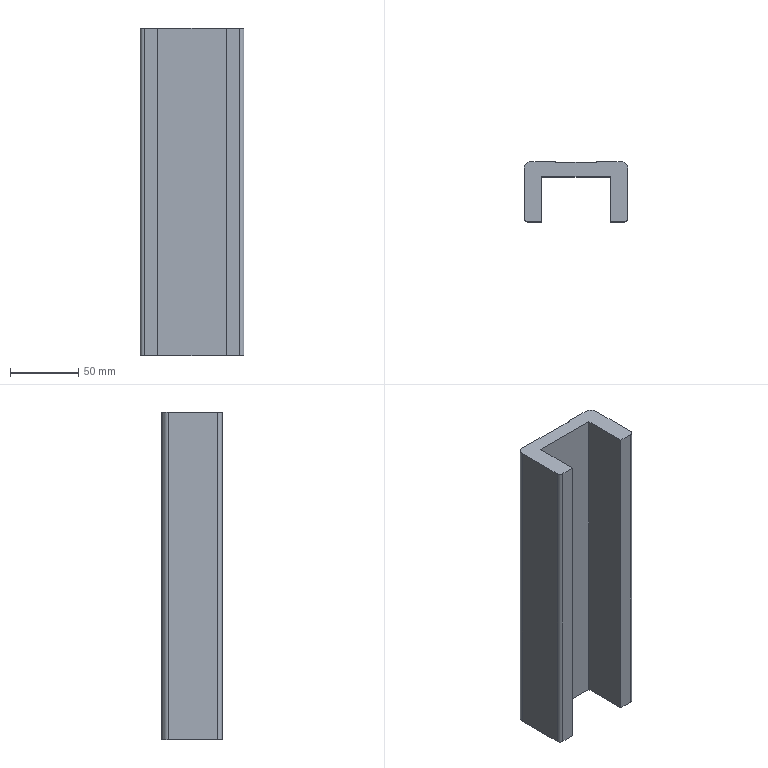Part | SolidWorks | features Cut 1, Extrusion 1 | 1 solid | 54 faces | box 76 x 44 x 240 mm | volume 396756 mm3 | cylinder 28 | plane 26 | commonest cylinder face diameters 5 x16 6 x10 10 x2
STEP:
#1=CARTESIAN_POINT('',(-22.,40.785,-167.));
#2=VERTEX_POINT('',#1);
#3=CARTESIAN_POINT('',(-28.,40.785,-167.));
#4=VERTEX_POINT('',#3);
#5=CARTESIAN_POINT('',(-25.,40.785,-167.));
#6=DIRECTION('',(0.,1.,0.));
#7=DIRECTION('',(-1.,0.,0.));
#8=AXIS2_PLACEMENT_3D('',#5,#6,#7);
#9=CIRCLE('',#8,3.);
#10=EDGE_CURVE('',#2,#4,#9,.T.);
#11=ORIENTED_EDGE('',*,*,#10,.F.);
#12=CARTESIAN_POINT('',(-22.,50.785,-167.));
#13=VERTEX_POINT('',#12);
#14=CARTESIAN_POINT('',(-22.,40.785,-167.));
#15=DIRECTION('',(0.,1.,0.));
#16=VECTOR('',#15,1000.);
#17=LINE('',#14,#16);
#18=EDGE_CURVE('',#2,#13,#17,.T.);
#19=ORIENTED_EDGE('',*,*,#18,.T.);
#20=CARTESIAN_POINT('',(-28.,50.785,-167.));
#21=VERTEX_POINT('',#20);
#22=CARTESIAN_POINT('',(-25.,50.785,-167.));
#23=DIRECTION('',(0.,1.,0.));
#24=DIRECTION('',(-1.,0.,0.));
#25=AXIS2_PLACEMENT_3D('',#22,#23,#24);
#26=CIRCLE('',#25,3.);
#27=EDGE_CURVE('',#13,#21,#26,.T.);
#28=ORIENTED_EDGE('',*,*,#27,.T.);
#29=CARTESIAN_POINT('',(-28.,40.785,-167.));
#30=DIRECTION('',(0.,1.,0.));
#31=VECTOR('',#30,1000.);
#32=LINE('',#29,#31);
#33=EDGE_CURVE('',#4,#21,#32,.T.);
#34=ORIENTED_EDGE('',*,*,#33,.F.);
#35=EDGE_LOOP('',(#11,#19,#28,#34));
#36=FACE_OUTER_BOUND('',#35,.T.);
#37=CARTESIAN_POINT('',(-25.,40.785,-167.));
#38=DIRECTION('',(0.,1.,0.));
#39=DIRECTION('',(-1.,0.,0.));
#40=AXIS2_PLACEMENT_3D('',#37,#38,#39);
#41=CYLINDRICAL_SURFACE('',#40,3.);
#42=ADVANCED_FACE('',(#36),#41,.F.);
#43=CARTESIAN_POINT('',(28.,40.785,-167.));
#44=VERTEX_POINT('',#43);
#45=CARTESIAN_POINT('',(22.,40.785,-167.));
#46=VERTEX_POINT('',#45);
#47=CARTESIAN_POINT('',(25.,40.785,-167.));
#48=DIRECTION('',(0.,1.,0.));
#49=DIRECTION('',(-1.,0.,0.));
#50=AXIS2_PLACEMENT_3D('',#47,#48,#49);
#51=CIRCLE('',#50,3.);
#52=EDGE_CURVE('',#44,#46,#51,.T.);
#53=ORIENTED_EDGE('',*,*,#52,.F.);
#54=CARTESIAN_POINT('',(28.,50.785,-167.));
#55=VERTEX_POINT('',#54);
#56=CARTESIAN_POINT('',(28.,40.785,-167.));
#57=DIRECTION('',(0.,1.,0.));
#58=VECTOR('',#57,1000.);
#59=LINE('',#56,#58);
#60=EDGE_CURVE('',#44,#55,#59,.T.);
#61=ORIENTED_EDGE('',*,*,#60,.T.);
#62=CARTESIAN_POINT('',(22.,50.785,-167.));
#63=VERTEX_POINT('',#62);
#64=CARTESIAN_POINT('',(25.,50.785,-167.));
#65=DIRECTION('',(0.,1.,0.));
#66=DIRECTION('',(-1.,0.,0.));
#67=AXIS2_PLACEMENT_3D('',#64,#65,#66);
#68=CIRCLE('',#67,3.);
#69=EDGE_CURVE('',#55,#63,#68,.T.);
#70=ORIENTED_EDGE('',*,*,#69,.T.);
#71=CARTESIAN_POINT('',(22.,40.785,-167.));
#72=DIRECTION('',(0.,1.,0.));
#73=VECTOR('',#72,1000.);
#74=LINE('',#71,#73);
#75=EDGE_CURVE('',#46,#63,#74,.T.);
#76=ORIENTED_EDGE('',*,*,#75,.F.);
#77=EDGE_LOOP('',(#53,#61,#70,#76));
#78=FACE_OUTER_BOUND('',#77,.T.);
#79=CARTESIAN_POINT('',(25.,40.785,-167.));
#80=DIRECTION('',(0.,1.,0.));
#81=DIRECTION('',(-1.,0.,0.));
#82=AXIS2_PLACEMENT_3D('',#79,#80,#81);
#83=CYLINDRICAL_SURFACE('',#82,3.);
#84=ADVANCED_FACE('',(#78),#83,.F.);
#85=CARTESIAN_POINT('',(-22.,40.785,-73.));
#86=VERTEX_POINT('',#85);
#87=CARTESIAN_POINT('',(-28.,40.785,-73.));
#88=VERTEX_POINT('',#87);
#89=CARTESIAN_POINT('',(-25.,40.785,-73.));
#90=DIRECTION('',(0.,1.,0.));
#91=DIRECTION('',(-1.,0.,0.));
#92=AXIS2_PLACEMENT_3D('',#89,#90,#91);
#93=CIRCLE('',#92,3.);
#94=EDGE_CURVE('',#86,#88,#93,.T.);
#95=ORIENTED_EDGE('',*,*,#94,.F.);
#96=CARTESIAN_POINT('',(-22.,50.785,-73.));
#97=VERTEX_POINT('',#96);
#98=CARTESIAN_POINT('',(-22.,40.785,-73.));
#99=DIRECTION('',(0.,1.,0.));
#100=VECTOR('',#99,1000.);
#101=LINE('',#98,#100);
#102=EDGE_CURVE('',#86,#97,#101,.T.);
#103=ORIENTED_EDGE('',*,*,#102,.T.);
#104=CARTESIAN_POINT('',(-28.,50.785,-73.));
#105=VERTEX_POINT('',#104);
#106=CARTESIAN_POINT('',(-25.,50.785,-73.));
#107=DIRECTION('',(0.,1.,0.));
#108=DIRECTION('',(-1.,0.,0.));
#109=AXIS2_PLACEMENT_3D('',#106,#107,#108);
#110=CIRCLE('',#109,3.);
#111=EDGE_CURVE('',#97,#105,#110,.T.);
#112=ORIENTED_EDGE('',*,*,#111,.T.);
#113=CARTESIAN_POINT('',(-28.,40.785,-73.));
#114=DIRECTION('',(0.,1.,0.));
#115=VECTOR('',#114,1000.);
#116=LINE('',#113,#115);
#117=EDGE_CURVE('',#88,#105,#116,.T.);
#118=ORIENTED_EDGE('',*,*,#117,.F.);
#119=EDGE_LOOP('',(#95,#103,#112,#118));
#120=FACE_OUTER_BOUND('',#119,.T.);
#121=CARTESIAN_POINT('',(-25.,40.785,-73.));
#122=DIRECTION('',(0.,1.,0.));
#123=DIRECTION('',(-1.,0.,0.));
#124=AXIS2_PLACEMENT_3D('',#121,#122,#123);
#125=CYLINDRICAL_SURFACE('',#124,3.);
#126=ADVANCED_FACE('',(#120),#125,.F.);
#127=CARTESIAN_POINT('',(-17.5,40.785,-216.));
#128=VERTEX_POINT('',#127);
#129=CARTESIAN_POINT('',(-22.5,40.785,-216.));
#130=VERTEX_POINT('',#129);
#131=CARTESIAN_POINT('',(-20.,40.785,-216.));
#132=DIRECTION('',(0.,1.,0.));
#133=DIRECTION('',(-1.,0.,0.));
#134=AXIS2_PLACEMENT_3D('',#131,#132,#133);
#135=CIRCLE('',#134,2.5);
#136=EDGE_CURVE('',#128,#130,#135,.T.);
#137=ORIENTED_EDGE('',*,*,#136,.F.);
#138=CARTESIAN_POINT('',(-17.5,50.785,-216.));
#139=VERTEX_POINT('',#138);
#140=CARTESIAN_POINT('',(-17.5,40.785,-216.));
#141=DIRECTION('',(0.,1.,0.));
#142=VECTOR('',#141,1000.);
#143=LINE('',#140,#142);
#144=EDGE_CURVE('',#128,#139,#143,.T.);
#145=ORIENTED_EDGE('',*,*,#144,.T.);
#146=CARTESIAN_POINT('',(-22.5,50.785,-216.));
#147=VERTEX_POINT('',#146);
#148=CARTESIAN_POINT('',(-20.,50.785,-216.));
#149=DIRECTION('',(0.,1.,0.));
#150=DIRECTION('',(-1.,0.,0.));
#151=AXIS2_PLACEMENT_3D('',#148,#149,#150);
#152=CIRCLE('',#151,2.5);
#153=EDGE_CURVE('',#139,#147,#152,.T.);
#154=ORIENTED_EDGE('',*,*,#153,.T.);
#155=CARTESIAN_POINT('',(-22.5,40.785,-216.));
#156=DIRECTION('',(0.,1.,0.));
#157=VECTOR('',#156,1000.);
#158=LINE('',#155,#157);
#159=EDGE_CURVE('',#130,#147,#158,.T.);
#160=ORIENTED_EDGE('',*,*,#159,.F.);
#161=EDGE_LOOP('',(#137,#145,#154,#160));
#162=FACE_OUTER_BOUND('',#161,.T.);
#163=CARTESIAN_POINT('',(-20.,40.785,-216.));
#164=DIRECTION('',(0.,1.,0.));
#165=DIRECTION('',(-1.,0.,0.));
#166=AXIS2_PLACEMENT_3D('',#163,#164,#165);
#167=CYLINDRICAL_SURFACE('',#166,2.5);
#168=ADVANCED_FACE('',(#162),#167,.F.);
#169=CARTESIAN_POINT('',(22.5,40.785,-216.));
#170=VERTEX_POINT('',#169);
#171=CARTESIAN_POINT('',(17.5,40.785,-216.));
#172=VERTEX_POINT('',#171);
#173=CARTESIAN_POINT('',(20.,40.785,-216.));
#174=DIRECTION('',(0.,1.,0.));
#175=DIRECTION('',(-1.,0.,0.));
#176=AXIS2_PLACEMENT_3D('',#173,#174,#175);
#177=CIRCLE('',#176,2.5);
#178=EDGE_CURVE('',#170,#172,#177,.T.);
#179=ORIENTED_EDGE('',*,*,#178,.F.);
#180=CARTESIAN_POINT('',(22.5,50.785,-216.));
#181=VERTEX_POINT('',#180);
#182=CARTESIAN_POINT('',(22.5,40.785,-216.));
#183=DIRECTION('',(0.,1.,0.));
#184=VECTOR('',#183,1000.);
#185=LINE('',#182,#184);
#186=EDGE_CURVE('',#170,#181,#185,.T.);
#187=ORIENTED_EDGE('',*,*,#186,.T.);
#188=CARTESIAN_POINT('',(17.5,50.785,-216.));
#189=VERTEX_POINT('',#188);
#190=CARTESIAN_POINT('',(20.,50.785,-216.));
#191=DIRECTION('',(0.,1.,0.));
#192=DIRECTION('',(-1.,0.,0.));
#193=AXIS2_PLACEMENT_3D('',#190,#191,#192);
#194=CIRCLE('',#193,2.5);
#195=EDGE_CURVE('',#181,#189,#194,.T.);
#196=ORIENTED_EDGE('',*,*,#195,.T.);
#197=CARTESIAN_POINT('',(17.5,40.785,-216.));
#198=DIRECTION('',(0.,1.,0.));
#199=VECTOR('',#198,1000.);
#200=LINE('',#197,#199);
#201=EDGE_CURVE('',#172,#189,#200,.T.);
#202=ORIENTED_EDGE('',*,*,#201,.F.);
#203=EDGE_LOOP('',(#179,#187,#196,#202));
#204=FACE_OUTER_BOUND('',#203,.T.);
#205=CARTESIAN_POINT('',(20.,40.785,-216.));
#206=DIRECTION('',(0.,1.,0.));
#207=DIRECTION('',(-1.,0.,0.));
#208=AXIS2_PLACEMENT_3D('',#205,#206,#207);
#209=CYLINDRICAL_SURFACE('',#208,2.5);
#210=ADVANCED_FACE('',(#204),#209,.F.);
#211=CARTESIAN_POINT('',(-17.5,40.785,-152.));
#212=VERTEX_POINT('',#211);
#213=CARTESIAN_POINT('',(-22.5,40.785,-152.));
#214=VERTEX_POINT('',#213);
#215=CARTESIAN_POINT('',(-20.,40.785,-152.));
#216=DIRECTION('',(0.,1.,0.));
#217=DIRECTION('',(-1.,0.,0.));
#218=AXIS2_PLACEMENT_3D('',#215,#216,#217);
#219=CIRCLE('',#218,2.5);
#220=EDGE_CURVE('',#212,#214,#219,.T.);
#221=ORIENTED_EDGE('',*,*,#220,.F.);
#222=CARTESIAN_POINT('',(-17.5,50.785,-152.));
#223=VERTEX_POINT('',#222);
#224=CARTESIAN_POINT('',(-17.5,40.785,-152.));
#225=DIRECTION('',(0.,1.,0.));
#226=VECTOR('',#225,1000.);
#227=LINE('',#224,#226);
#228=EDGE_CURVE('',#212,#223,#227,.T.);
#229=ORIENTED_EDGE('',*,*,#228,.T.);
#230=CARTESIAN_POINT('',(-22.5,50.785,-152.));
#231=VERTEX_POINT('',#230);
#232=CARTESIAN_POINT('',(-20.,50.785,-152.));
#233=DIRECTION('',(0.,1.,0.));
#234=DIRECTION('',(-1.,0.,0.));
#235=AXIS2_PLACEMENT_3D('',#232,#233,#234);
#236=CIRCLE('',#235,2.5);
#237=EDGE_CURVE('',#223,#231,#236,.T.);
#238=ORIENTED_EDGE('',*,*,#237,.T.);
#239=CARTESIAN_POINT('',(-22.5,40.785,-152.));
#240=DIRECTION('',(0.,1.,0.));
#241=VECTOR('',#240,1000.);
#242=LINE('',#239,#241);
#243=EDGE_CURVE('',#214,#231,#242,.T.);
#244=ORIENTED_EDGE('',*,*,#243,.F.);
#245=EDGE_LOOP('',(#221,#229,#238,#244));
#246=FACE_OUTER_BOUND('',#245,.T.);
#247=CARTESIAN_POINT('',(-20.,40.785,-152.));
#248=DIRECTION('',(0.,1.,0.));
#249=DIRECTION('',(-1.,0.,0.));
#250=AXIS2_PLACEMENT_3D('',#247,#248,#249);
#251=CYLINDRICAL_SURFACE('',#250,2.5);
#252=ADVANCED_FACE('',(#246),#251,.F.);
#253=CARTESIAN_POINT('',(22.5,40.785,-152.));
#254=VERTEX_POINT('',#253);
#255=CARTESIAN_POINT('',(17.5,40.785,-152.));
#256=VERTEX_POINT('',#255);
#257=CARTESIAN_POINT('',(20.,40.785,-152.));
#258=DIRECTION('',(0.,1.,0.));
#259=DIRECTION('',(-1.,0.,0.));
#260=AXIS2_PLACEMENT_3D('',#257,#258,#259);
#261=CIRCLE('',#260,2.5);
#262=EDGE_CURVE('',#254,#256,#261,.T.);
#263=ORIENTED_EDGE('',*,*,#262,.F.);
#264=CARTESIAN_POINT('',(22.5,50.785,-152.));
#265=VERTEX_POINT('',#264);
#266=CARTESIAN_POINT('',(22.5,40.785,-152.));
#267=DIRECTION('',(0.,1.,0.));
#268=VECTOR('',#267,1000.);
#269=LINE('',#266,#268);
#270=EDGE_CURVE('',#254,#265,#269,.T.);
#271=ORIENTED_EDGE('',*,*,#270,.T.);
#272=CARTESIAN_POINT('',(17.5,50.785,-152.));
#273=VERTEX_POINT('',#272);
#274=CARTESIAN_POINT('',(20.,50.785,-152.));
#275=DIRECTION('',(0.,1.,0.));
#276=DIRECTION('',(-1.,0.,0.));
#277=AXIS2_PLACEMENT_3D('',#274,#275,#276);
#278=CIRCLE('',#277,2.5);
#279=EDGE_CURVE('',#265,#273,#278,.T.);
#280=ORIENTED_EDGE('',*,*,#279,.T.);
#281=CARTESIAN_POINT('',(17.5,40.785,-152.));
#282=DIRECTION('',(0.,1.,0.));
#283=VECTOR('',#282,1000.);
#284=LINE('',#281,#283);
#285=EDGE_CURVE('',#256,#273,#284,.T.);
#286=ORIENTED_EDGE('',*,*,#285,.F.);
#287=EDGE_LOOP('',(#263,#271,#280,#286));
#288=FACE_OUTER_BOUND('',#287,.T.);
#289=CARTESIAN_POINT('',(20.,40.785,-152.));
#290=DIRECTION('',(0.,1.,0.));
#291=DIRECTION('',(-1.,0.,0.));
#292=AXIS2_PLACEMENT_3D('',#289,#290,#291);
#293=CYLINDRICAL_SURFACE('',#292,2.5);
#294=ADVANCED_FACE('',(#288),#293,.F.);
#295=CARTESIAN_POINT('',(-17.5,40.785,-88.));
#296=VERTEX_POINT('',#295);
#297=CARTESIAN_POINT('',(-22.5,40.785,-88.));
#298=VERTEX_POINT('',#297);
#299=CARTESIAN_POINT('',(-20.,40.785,-88.));
#300=DIRECTION('',(0.,1.,0.));
#301=DIRECTION('',(-1.,0.,0.));
#302=AXIS2_PLACEMENT_3D('',#299,#300,#301);
#303=CIRCLE('',#302,2.5);
#304=EDGE_CURVE('',#296,#298,#303,.T.);
#305=ORIENTED_EDGE('',*,*,#304,.F.);
#306=CARTESIAN_POINT('',(-17.5,50.785,-88.));
#307=VERTEX_POINT('',#306);
#308=CARTESIAN_POINT('',(-17.5,40.785,-88.));
#309=DIRECTION('',(0.,1.,0.));
#310=VECTOR('',#309,1000.);
#311=LINE('',#308,#310);
#312=EDGE_CURVE('',#296,#307,#311,.T.);
#313=ORIENTED_EDGE('',*,*,#312,.T.);
#314=CARTESIAN_POINT('',(-22.5,50.785,-88.));
#315=VERTEX_POINT('',#314);
#316=CARTESIAN_POINT('',(-20.,50.785,-88.));
#317=DIRECTION('',(0.,1.,0.));
#318=DIRECTION('',(-1.,0.,0.));
#319=AXIS2_PLACEMENT_3D('',#316,#317,#318);
#320=CIRCLE('',#319,2.5);
#321=EDGE_CURVE('',#307,#315,#320,.T.);
#322=ORIENTED_EDGE('',*,*,#321,.T.);
#323=CARTESIAN_POINT('',(-22.5,40.785,-88.));
#324=DIRECTION('',(0.,1.,0.));
#325=VECTOR('',#324,1000.);
#326=LINE('',#323,#325);
#327=EDGE_CURVE('',#298,#315,#326,.T.);
#328=ORIENTED_EDGE('',*,*,#327,.F.);
#329=EDGE_LOOP('',(#305,#313,#322,#328));
#330=FACE_OUTER_BOUND('',#329,.T.);
#331=CARTESIAN_POINT('',(-20.,40.785,-88.));
#332=DIRECTION('',(0.,1.,0.));
#333=DIRECTION('',(-1.,0.,0.));
#334=AXIS2_PLACEMENT_3D('',#331,#332,#333);
#335=CYLINDRICAL_SURFACE('',#334,2.5);
#336=ADVANCED_FACE('',(#330),#335,.F.);
#337=CARTESIAN_POINT('',(22.5,40.785,-88.));
#338=VERTEX_POINT('',#337);
#339=CARTESIAN_POINT('',(17.5,40.785,-88.));
#340=VERTEX_POINT('',#339);
#341=CARTESIAN_POINT('',(20.,40.785,-88.));
#342=DIRECTION('',(0.,1.,0.));
#343=DIRECTION('',(-1.,0.,0.));
#344=AXIS2_PLACEMENT_3D('',#341,#342,#343);
#345=CIRCLE('',#344,2.5);
#346=EDGE_CURVE('',#338,#340,#345,.T.);
#347=ORIENTED_EDGE('',*,*,#346,.F.);
#348=CARTESIAN_POINT('',(22.5,50.785,-88.));
#349=VERTEX_POINT('',#348);
#350=CARTESIAN_POINT('',(22.5,40.785,-88.));
#351=DIRECTION('',(0.,1.,0.));
#352=VECTOR('',#351,1000.);
#353=LINE('',#350,#352);
#354=EDGE_CURVE('',#338,#349,#353,.T.);
#355=ORIENTED_EDGE('',*,*,#354,.T.);
#356=CARTESIAN_POINT('',(17.5,50.785,-88.));
#357=VERTEX_POINT('',#356);
#358=CARTESIAN_POINT('',(20.,50.785,-88.));
#359=DIRECTION('',(0.,1.,0.));
#360=DIRECTION('',(-1.,0.,0.));
#361=AXIS2_PLACEMENT_3D('',#358,#359,#360);
#362=CIRCLE('',#361,2.5);
#363=EDGE_CURVE('',#349,#357,#362,.T.);
#364=ORIENTED_EDGE('',*,*,#363,.T.);
#365=CARTESIAN_POINT('',(17.5,40.785,-88.));
#366=DIRECTION('',(0.,1.,0.));
#367=VECTOR('',#366,1000.);
#368=LINE('',#365,#367);
#369=EDGE_CURVE('',#340,#357,#368,.T.);
#370=ORIENTED_EDGE('',*,*,#369,.F.);
#371=EDGE_LOOP('',(#347,#355,#364,#370));
#372=FACE_OUTER_BOUND('',#371,.T.);
#373=CARTESIAN_POINT('',(20.,40.785,-88.));
#374=DIRECTION('',(0.,1.,0.));
#375=DIRECTION('',(-1.,0.,0.));
#376=AXIS2_PLACEMENT_3D('',#373,#374,#375);
#377=CYLINDRICAL_SURFACE('',#376,2.5);
#378=ADVANCED_FACE('',(#372),#377,.F.);
#379=CARTESIAN_POINT('',(-17.5,40.785,-24.));
#380=VERTEX_POINT('',#379);
#381=CARTESIAN_POINT('',(-22.5,40.785,-24.));
#382=VERTEX_POINT('',#381);
#383=CARTESIAN_POINT('',(-20.,40.785,-24.));
#384=DIRECTION('',(0.,1.,0.));
#385=DIRECTION('',(-1.,0.,0.));
#386=AXIS2_PLACEMENT_3D('',#383,#384,#385);
#387=CIRCLE('',#386,2.5);
#388=EDGE_CURVE('',#380,#382,#387,.T.);
#389=ORIENTED_EDGE('',*,*,#388,.F.);
#390=CARTESIAN_POINT('',(-17.5,50.785,-24.));
#391=VERTEX_POINT('',#390);
#392=CARTESIAN_POINT('',(-17.5,40.785,-24.));
#393=DIRECTION('',(0.,1.,0.));
#394=VECTOR('',#393,1000.);
#395=LINE('',#392,#394);
#396=EDGE_CURVE('',#380,#391,#395,.T.);
#397=ORIENTED_EDGE('',*,*,#396,.T.);
#398=CARTESIAN_POINT('',(-22.5,50.785,-24.));
#399=VERTEX_POINT('',#398);
#400=CARTESIAN_POINT('',(-20.,50.785,-24.));
#401=DIRECTION('',(0.,1.,0.));
#402=DIRECTION('',(-1.,0.,0.));
#403=AXIS2_PLACEMENT_3D('',#400,#401,#402);
#404=CIRCLE('',#403,2.5);
#405=EDGE_CURVE('',#391,#399,#404,.T.);
#406=ORIENTED_EDGE('',*,*,#405,.T.);
#407=CARTESIAN_POINT('',(-22.5,40.785,-24.));
#408=DIRECTION('',(0.,1.,0.));
#409=VECTOR('',#408,1000.);
#410=LINE('',#407,#409);
#411=EDGE_CURVE('',#382,#399,#410,.T.);
#412=ORIENTED_EDGE('',*,*,#411,.F.);
#413=EDGE_LOOP('',(#389,#397,#406,#412));
#414=FACE_OUTER_BOUND('',#413,.T.);
#415=CARTESIAN_POINT('',(-20.,40.785,-24.));
#416=DIRECTION('',(0.,1.,0.));
#417=DIRECTION('',(-1.,0.,0.));
#418=AXIS2_PLACEMENT_3D('',#415,#416,#417);
#419=CYLINDRICAL_SURFACE('',#418,2.5);
#420=ADVANCED_FACE('',(#414),#419,.F.);
#421=CARTESIAN_POINT('',(28.,40.785,-73.));
#422=VERTEX_POINT('',#421);
#423=CARTESIAN_POINT('',(22.,40.785,-73.));
#424=VERTEX_POINT('',#423);
#425=CARTESIAN_POINT('',(25.,40.785,-73.));
#426=DIRECTION('',(0.,1.,0.));
#427=DIRECTION('',(-1.,0.,0.));
#428=AXIS2_PLACEMENT_3D('',#425,#426,#427);
#429=CIRCLE('',#428,3.);
#430=EDGE_CURVE('',#422,#424,#429,.T.);
#431=ORIENTED_EDGE('',*,*,#430,.F.);
#432=CARTESIAN_POINT('',(28.,50.785,-73.));
#433=VERTEX_POINT('',#432);
#434=CARTESIAN_POINT('',(28.,40.785,-73.));
#435=DIRECTION('',(0.,1.,0.));
#436=VECTOR('',#435,1000.);
#437=LINE('',#434,#436);
#438=EDGE_CURVE('',#422,#433,#437,.T.);
#439=ORIENTED_EDGE('',*,*,#438,.T.);
#440=CARTESIAN_POINT('',(22.,50.785,-73.));
#441=VERTEX_POINT('',#440);
#442=CARTESIAN_POINT('',(25.,50.785,-73.));
#443=DIRECTION('',(0.,1.,0.));
#444=DIRECTION('',(-1.,0.,0.));
#445=AXIS2_PLACEMENT_3D('',#442,#443,#444);
#446=CIRCLE('',#445,3.);
#447=EDGE_CURVE('',#433,#441,#446,.T.);
#448=ORIENTED_EDGE('',*,*,#447,.T.);
#449=CARTESIAN_POINT('',(22.,40.785,-73.));
#450=DIRECTION('',(0.,1.,0.));
#451=VECTOR('',#450,1000.);
#452=LINE('',#449,#451);
#453=EDGE_CURVE('',#424,#441,#452,.T.);
#454=ORIENTED_EDGE('',*,*,#453,.F.);
#455=EDGE_LOOP('',(#431,#439,#448,#454));
#456=FACE_OUTER_BOUND('',#455,.T.);
#457=CARTESIAN_POINT('',(25.,40.785,-73.));
#458=DIRECTION('',(0.,1.,0.));
#459=DIRECTION('',(-1.,0.,0.));
#460=AXIS2_PLACEMENT_3D('',#457,#458,#459);
#461=CYLINDRICAL_SURFACE('',#460,3.);
#462=ADVANCED_FACE('',(#456),#461,.F.);
#463=CARTESIAN_POINT('',(22.5,40.785,-24.));
#464=VERTEX_POINT('',#463);
#465=CARTESIAN_POINT('',(17.5,40.785,-24.));
#466=VERTEX_POINT('',#465);
#467=CARTESIAN_POINT('',(20.,40.785,-24.));
#468=DIRECTION('',(0.,1.,0.));
#469=DIRECTION('',(-1.,0.,0.));
#470=AXIS2_PLACEMENT_3D('',#467,#468,#469);
#471=CIRCLE('',#470,2.5);
#472=EDGE_CURVE('',#464,#466,#471,.T.);
#473=ORIENTED_EDGE('',*,*,#472,.F.);
#474=CARTESIAN_POINT('',(22.5,50.785,-24.));
#475=VERTEX_POINT('',#474);
#476=CARTESIAN_POINT('',(22.5,40.785,-24.));
#477=DIRECTION('',(0.,1.,0.));
#478=VECTOR('',#477,1000.);
#479=LINE('',#476,#478);
#480=EDGE_CURVE('',#464,#475,#479,.T.);
#481=ORIENTED_EDGE('',*,*,#480,.T.);
#482=CARTESIAN_POINT('',(17.5,50.785,-24.));
#483=VERTEX_POINT('',#482);
#484=CARTESIAN_POINT('',(20.,50.785,-24.));
#485=DIRECTION('',(0.,1.,0.));
#486=DIRECTION('',(-1.,0.,0.));
#487=AXIS2_PLACEMENT_3D('',#484,#485,#486);
#488=CIRCLE('',#487,2.5);
#489=EDGE_CURVE('',#475,#483,#488,.T.);
#490=ORIENTED_EDGE('',*,*,#489,.T.);
#491=CARTESIAN_POINT('',(17.5,40.785,-24.));
#492=DIRECTION('',(0.,1.,0.));
#493=VECTOR('',#492,1000.);
#494=LINE('',#491,#493);
#495=EDGE_CURVE('',#466,#483,#494,.T.);
#496=ORIENTED_EDGE('',*,*,#495,.F.);
#497=EDGE_LOOP('',(#473,#481,#490,#496));
#498=FACE_OUTER_BOUND('',#497,.T.);
#499=CARTESIAN_POINT('',(20.,40.785,-24.));
#500=DIRECTION('',(0.,1.,0.));
#501=DIRECTION('',(-1.,0.,0.));
#502=AXIS2_PLACEMENT_3D('',#499,#500,#501);
#503=CYLINDRICAL_SURFACE('',#502,2.5);
#504=ADVANCED_FACE('',(#498),#503,.F.);
#505=CARTESIAN_POINT('',(-25.,50.785,-167.));
#506=DIRECTION('',(0.,1.,0.));
#507=DIRECTION('',(-1.,0.,0.));
#508=AXIS2_PLACEMENT_3D('',#505,#506,#507);
#509=CIRCLE('',#508,3.);
#510=EDGE_CURVE('',#21,#13,#509,.T.);
#511=ORIENTED_EDGE('',*,*,#510,.F.);
#512=ORIENTED_EDGE('',*,*,#27,.F.);
#513=EDGE_LOOP('',(#511,#512));
#514=FACE_BOUND('',#513,.T.);
#515=CARTESIAN_POINT('',(-25.,50.785,-73.));
#516=DIRECTION('',(0.,1.,0.));
#517=DIRECTION('',(-1.,0.,0.));
#518=AXIS2_PLACEMENT_3D('',#515,#516,#517);
#519=CIRCLE('',#518,3.);
#520=EDGE_CURVE('',#105,#97,#519,.T.);
#521=ORIENTED_EDGE('',*,*,#520,.F.);
#522=ORIENTED_EDGE('',*,*,#111,.F.);
#523=EDGE_LOOP('',(#521,#522));
#524=FACE_BOUND('',#523,.T.);
#525=CARTESIAN_POINT('',(-20.,50.785,-216.));
#526=DIRECTION('',(0.,1.,0.));
#527=DIRECTION('',(-1.,0.,0.));
#528=AXIS2_PLACEMENT_3D('',#525,#526,#527);
#529=CIRCLE('',#528,2.5);
#530=EDGE_CURVE('',#147,#139,#529,.T.);
#531=ORIENTED_EDGE('',*,*,#530,.F.);
#532=ORIENTED_EDGE('',*,*,#153,.F.);
#533=EDGE_LOOP('',(#531,#532));
#534=FACE_BOUND('',#533,.T.);
#535=CARTESIAN_POINT('',(-20.,50.785,-152.));
#536=DIRECTION('',(0.,1.,0.));
#537=DIRECTION('',(-1.,0.,0.));
#538=AXIS2_PLACEMENT_3D('',#535,#536,#537);
#539=CIRCLE('',#538,2.5);
#540=EDGE_CURVE('',#231,#223,#539,.T.);
#541=ORIENTED_EDGE('',*,*,#540,.F.);
#542=ORIENTED_EDGE('',*,*,#237,.F.);
#543=EDGE_LOOP('',(#541,#542));
#544=FACE_BOUND('',#543,.T.);
#545=CARTESIAN_POINT('',(-20.,50.785,-88.));
#546=DIRECTION('',(0.,1.,0.));
#547=DIRECTION('',(-1.,0.,0.));
#548=AXIS2_PLACEMENT_3D('',#545,#546,#547);
#549=CIRCLE('',#548,2.5);
#550=EDGE_CURVE('',#315,#307,#549,.T.);
#551=ORIENTED_EDGE('',*,*,#550,.F.);
#552=ORIENTED_EDGE('',*,*,#321,.F.);
#553=EDGE_LOOP('',(#551,#552));
#554=FACE_BOUND('',#553,.T.);
#555=CARTESIAN_POINT('',(-20.,50.785,-24.));
#556=DIRECTION('',(0.,1.,0.));
#557=DIRECTION('',(-1.,0.,0.));
#558=AXIS2_PLACEMENT_3D('',#555,#556,#557);
#559=CIRCLE('',#558,2.5);
#560=EDGE_CURVE('',#399,#391,#559,.T.);
#561=ORIENTED_EDGE('',*,*,#560,.F.);
#562=ORIENTED_EDGE('',*,*,#405,.F.);
#563=EDGE_LOOP('',(#561,#562));
#564=FACE_BOUND('',#563,.T.);
#565=CARTESIAN_POINT('',(-15.,50.785,0.));
#566=VERTEX_POINT('',#565);
#567=CARTESIAN_POINT('',(-33.,50.785,0.));
#568=VERTEX_POINT('',#567);
#569=CARTESIAN_POINT('',(-15.,50.785,0.));
#570=DIRECTION('',(-1.,0.,0.));
#571=VECTOR('',#570,1000.);
#572=LINE('',#569,#571);
#573=EDGE_CURVE('',#566,#568,#572,.T.);
#574=ORIENTED_EDGE('',*,*,#573,.F.);
#575=CARTESIAN_POINT('',(-15.,50.785,-240.));
#576=VERTEX_POINT('',#575);
#577=CARTESIAN_POINT('',(-15.,50.785,-240.));
#578=DIRECTION('',(0.,0.,1.));
#579=VECTOR('',#578,1000.);
#580=LINE('',#577,#579);
#581=EDGE_CURVE('',#576,#566,#580,.T.);
#582=ORIENTED_EDGE('',*,*,#581,.F.);
#583=CARTESIAN_POINT('',(-33.,50.785,-240.));
#584=VERTEX_POINT('',#583);
#585=CARTESIAN_POINT('',(-15.,50.785,-240.));
#586=DIRECTION('',(-1.,0.,0.));
#587=VECTOR('',#586,1000.);
#588=LINE('',#585,#587);
#589=EDGE_CURVE('',#576,#584,#588,.T.);
#590=ORIENTED_EDGE('',*,*,#589,.T.);
#591=CARTESIAN_POINT('',(-33.,50.785,-240.));
#592=DIRECTION('',(0.,0.,1.));
#593=VECTOR('',#592,1000.);
#594=LINE('',#591,#593);
#595=EDGE_CURVE('',#584,#568,#594,.T.);
#596=ORIENTED_EDGE('',*,*,#595,.T.);
#597=EDGE_LOOP('',(#574,#582,#590,#596));
#598=FACE_OUTER_BOUND('',#597,.T.);
#599=CARTESIAN_POINT('',(-15.,50.785,-240.));
#600=DIRECTION('',(0.,1.,0.));
#601=DIRECTION('',(-1.,0.,0.));
#602=AXIS2_PLACEMENT_3D('',#599,#600,#601);
#603=PLANE('',#602);
#604=ADVANCED_FACE('',(#514,#524,#534,#544,#554,#564,#598),#603,.T.);
#605=CARTESIAN_POINT('',(-15.,50.285,0.));
#606=VERTEX_POINT('',#605);
#607=CARTESIAN_POINT('',(-15.,50.785,0.));
#608=DIRECTION('',(0.,1.,0.));
#609=VECTOR('',#608,1000.);
#610=LINE('',#607,#609);
#611=EDGE_CURVE('',#606,#566,#610,.T.);
#612=ORIENTED_EDGE('',*,*,#611,.F.);
#613=CARTESIAN_POINT('',(-15.,50.285,-240.));
#614=VERTEX_POINT('',#613);
#615=CARTESIAN_POINT('',(-15.,50.285,-240.));
#616=DIRECTION('',(0.,0.,1.));
#617=VECTOR('',#616,1000.);
#618=LINE('',#615,#617);
#619=EDGE_CURVE('',#614,#606,#618,.T.);
#620=ORIENTED_EDGE('',*,*,#619,.F.);
#621=CARTESIAN_POINT('',(-15.,50.785,-240.));
#622=DIRECTION('',(0.,1.,0.));
#623=VECTOR('',#622,1000.);
#624=LINE('',#621,#623);
#625=EDGE_CURVE('',#614,#576,#624,.T.);
#626=ORIENTED_EDGE('',*,*,#625,.T.);
#627=ORIENTED_EDGE('',*,*,#581,.T.);
#628=EDGE_LOOP('',(#612,#620,#626,#627));
#629=FACE_OUTER_BOUND('',#628,.T.);
#630=CARTESIAN_POINT('',(-15.,50.785,-240.));
#631=DIRECTION('',(1.,0.,0.));
#632=DIRECTION('',(0.,0.,-1.));
#633=AXIS2_PLACEMENT_3D('',#630,#631,#632);
#634=PLANE('',#633);
#635=ADVANCED_FACE('',(#629),#634,.T.);
#636=CARTESIAN_POINT('',(15.,50.285,0.));
#637=VERTEX_POINT('',#636);
#638=CARTESIAN_POINT('',(-15.,50.285,0.));
#639=DIRECTION('',(-1.,0.,0.));
#640=VECTOR('',#639,1000.);
#641=LINE('',#638,#640);
#642=EDGE_CURVE('',#637,#606,#641,.T.);
#643=ORIENTED_EDGE('',*,*,#642,.F.);
#644=CARTESIAN_POINT('',(15.,50.285,-240.));
#645=VERTEX_POINT('',#644);
#646=CARTESIAN_POINT('',(15.,50.285,-240.));
#647=DIRECTION('',(0.,0.,1.));
#648=VECTOR('',#647,1000.);
#649=LINE('',#646,#648);
#650=EDGE_CURVE('',#645,#637,#649,.T.);
#651=ORIENTED_EDGE('',*,*,#650,.F.);
#652=CARTESIAN_POINT('',(-15.,50.285,-240.));
#653=DIRECTION('',(-1.,0.,0.));
#654=VECTOR('',#653,1000.);
#655=LINE('',#652,#654);
#656=EDGE_CURVE('',#645,#614,#655,.T.);
#657=ORIENTED_EDGE('',*,*,#656,.T.);
#658=ORIENTED_EDGE('',*,*,#619,.T.);
#659=EDGE_LOOP('',(#643,#651,#657,#658));
#660=FACE_OUTER_BOUND('',#659,.T.);
#661=CARTESIAN_POINT('',(-15.,50.285,-240.));
#662=DIRECTION('',(0.,1.,0.));
#663=DIRECTION('',(0.,0.,1.));
#664=AXIS2_PLACEMENT_3D('',#661,#662,#663);
#665=PLANE('',#664);
#666=ADVANCED_FACE('',(#660),#665,.T.);
#667=CARTESIAN_POINT('',(15.,50.785,0.));
#668=VERTEX_POINT('',#667);
#669=CARTESIAN_POINT('',(15.,50.785,0.));
#670=DIRECTION('',(0.,-1.,0.));
#671=VECTOR('',#670,1000.);
#672=LINE('',#669,#671);
#673=EDGE_CURVE('',#668,#637,#672,.T.);
#674=ORIENTED_EDGE('',*,*,#673,.F.);
#675=CARTESIAN_POINT('',(15.,50.785,-240.));
#676=VERTEX_POINT('',#675);
#677=CARTESIAN_POINT('',(15.,50.785,-240.));
#678=DIRECTION('',(0.,0.,1.));
#679=VECTOR('',#678,1000.);
#680=LINE('',#677,#679);
#681=EDGE_CURVE('',#676,#668,#680,.T.);
#682=ORIENTED_EDGE('',*,*,#681,.F.);
#683=CARTESIAN_POINT('',(15.,50.785,-240.));
#684=DIRECTION('',(0.,-1.,0.));
#685=VECTOR('',#684,1000.);
#686=LINE('',#683,#685);
#687=EDGE_CURVE('',#676,#645,#686,.T.);
#688=ORIENTED_EDGE('',*,*,#687,.T.);
#689=ORIENTED_EDGE('',*,*,#650,.T.);
#690=EDGE_LOOP('',(#674,#682,#688,#689));
#691=FACE_OUTER_BOUND('',#690,.T.);
#692=CARTESIAN_POINT('',(15.,50.785,-240.));
#693=DIRECTION('',(-1.,0.,0.));
#694=DIRECTION('',(0.,0.,1.));
#695=AXIS2_PLACEMENT_3D('',#692,#693,#694);
#696=PLANE('',#695);
#697=ADVANCED_FACE('',(#691),#696,.T.);
#698=CARTESIAN_POINT('',(25.,50.785,-167.));
#699=DIRECTION('',(0.,1.,0.));
#700=DIRECTION('',(-1.,0.,0.));
#701=AXIS2_PLACEMENT_3D('',#698,#699,#700);
#702=CIRCLE('',#701,3.);
#703=EDGE_CURVE('',#63,#55,#702,.T.);
#704=ORIENTED_EDGE('',*,*,#703,.F.);
#705=ORIENTED_EDGE('',*,*,#69,.F.);
#706=EDGE_LOOP('',(#704,#705));
#707=FACE_BOUND('',#706,.T.);
#708=CARTESIAN_POINT('',(20.,50.785,-216.));
#709=DIRECTION('',(0.,1.,0.));
#710=DIRECTION('',(-1.,0.,0.));
#711=AXIS2_PLACEMENT_3D('',#708,#709,#710);
#712=CIRCLE('',#711,2.5);
#713=EDGE_CURVE('',#189,#181,#712,.T.);
#714=ORIENTED_EDGE('',*,*,#713,.F.);
#715=ORIENTED_EDGE('',*,*,#195,.F.);
#716=EDGE_LOOP('',(#714,#715));
#717=FACE_BOUND('',#716,.T.);
#718=CARTESIAN_POINT('',(20.,50.785,-152.));
#719=DIRECTION('',(0.,1.,0.));
#720=DIRECTION('',(-1.,0.,0.));
#721=AXIS2_PLACEMENT_3D('',#718,#719,#720);
#722=CIRCLE('',#721,2.5);
#723=EDGE_CURVE('',#273,#265,#722,.T.);
#724=ORIENTED_EDGE('',*,*,#723,.F.);
#725=ORIENTED_EDGE('',*,*,#279,.F.);
#726=EDGE_LOOP('',(#724,#725));
#727=FACE_BOUND('',#726,.T.);
#728=CARTESIAN_POINT('',(20.,50.785,-88.));
#729=DIRECTION('',(0.,1.,0.));
#730=DIRECTION('',(-1.,0.,0.));
#731=AXIS2_PLACEMENT_3D('',#728,#729,#730);
#732=CIRCLE('',#731,2.5);
#733=EDGE_CURVE('',#357,#349,#732,.T.);
#734=ORIENTED_EDGE('',*,*,#733,.F.);
#735=ORIENTED_EDGE('',*,*,#363,.F.);
#736=EDGE_LOOP('',(#734,#735));
#737=FACE_BOUND('',#736,.T.);
#738=CARTESIAN_POINT('',(25.,50.785,-73.));
#739=DIRECTION('',(0.,1.,0.));
#740=DIRECTION('',(-1.,0.,0.));
#741=AXIS2_PLACEMENT_3D('',#738,#739,#740);
#742=CIRCLE('',#741,3.);
#743=EDGE_CURVE('',#441,#433,#742,.T.);
#744=ORIENTED_EDGE('',*,*,#743,.F.);
#745=ORIENTED_EDGE('',*,*,#447,.F.);
#746=EDGE_LOOP('',(#744,#745));
#747=FACE_BOUND('',#746,.T.);
#748=CARTESIAN_POINT('',(20.,50.785,-24.));
#749=DIRECTION('',(0.,1.,0.));
#750=DIRECTION('',(-1.,0.,0.));
#751=AXIS2_PLACEMENT_3D('',#748,#749,#750);
#752=CIRCLE('',#751,2.5);
#753=EDGE_CURVE('',#483,#475,#752,.T.);
#754=ORIENTED_EDGE('',*,*,#753,.F.);
#755=ORIENTED_EDGE('',*,*,#489,.F.);
#756=EDGE_LOOP('',(#754,#755));
#757=FACE_BOUND('',#756,.T.);
#758=CARTESIAN_POINT('',(33.,50.785,0.));
#759=VERTEX_POINT('',#758);
#760=CARTESIAN_POINT('',(33.,50.785,0.));
#761=DIRECTION('',(-1.,0.,0.));
#762=VECTOR('',#761,1000.);
#763=LINE('',#760,#762);
#764=EDGE_CURVE('',#759,#668,#763,.T.);
#765=ORIENTED_EDGE('',*,*,#764,.F.);
#766=CARTESIAN_POINT('',(33.,50.785,-240.));
#767=VERTEX_POINT('',#766);
#768=CARTESIAN_POINT('',(33.,50.785,-240.));
#769=DIRECTION('',(0.,0.,1.));
#770=VECTOR('',#769,1000.);
#771=LINE('',#768,#770);
#772=EDGE_CURVE('',#767,#759,#771,.T.);
#773=ORIENTED_EDGE('',*,*,#772,.F.);
#774=CARTESIAN_POINT('',(33.,50.785,-240.));
#775=DIRECTION('',(-1.,0.,0.));
#776=VECTOR('',#775,1000.);
#777=LINE('',#774,#776);
#778=EDGE_CURVE('',#767,#676,#777,.T.);
#779=ORIENTED_EDGE('',*,*,#778,.T.);
#780=ORIENTED_EDGE('',*,*,#681,.T.);
#781=EDGE_LOOP('',(#765,#773,#779,#780));
#782=FACE_OUTER_BOUND('',#781,.T.);
#783=CARTESIAN_POINT('',(33.,50.785,-240.));
#784=DIRECTION('',(0.,1.,0.));
#785=DIRECTION('',(-1.,0.,0.));
#786=AXIS2_PLACEMENT_3D('',#783,#784,#785);
#787=PLANE('',#786);
#788=ADVANCED_FACE('',(#707,#717,#727,#737,#747,#757,#782),#787,.T.);
#789=CARTESIAN_POINT('',(38.,45.785,0.));
#790=VERTEX_POINT('',#789);
#791=CARTESIAN_POINT('',(33.,45.785,0.));
#792=DIRECTION('',(0.,0.,1.));
#793=DIRECTION('',(1.,0.,0.));
#794=AXIS2_PLACEMENT_3D('',#791,#792,#793);
#795=CIRCLE('',#794,5.);
#796=EDGE_CURVE('',#790,#759,#795,.T.);
#797=ORIENTED_EDGE('',*,*,#796,.F.);
#798=CARTESIAN_POINT('',(38.,45.785,-240.));
#799=VERTEX_POINT('',#798);
#800=CARTESIAN_POINT('',(38.,45.785,-240.));
#801=DIRECTION('',(0.,0.,1.));
#802=VECTOR('',#801,1000.);
#803=LINE('',#800,#802);
#804=EDGE_CURVE('',#799,#790,#803,.T.);
#805=ORIENTED_EDGE('',*,*,#804,.F.);
#806=CARTESIAN_POINT('',(33.,45.785,-240.));
#807=DIRECTION('',(0.,0.,1.));
#808=DIRECTION('',(1.,0.,0.));
#809=AXIS2_PLACEMENT_3D('',#806,#807,#808);
#810=CIRCLE('',#809,5.);
#811=EDGE_CURVE('',#799,#767,#810,.T.);
#812=ORIENTED_EDGE('',*,*,#811,.T.);
#813=ORIENTED_EDGE('',*,*,#772,.T.);
#814=EDGE_LOOP('',(#797,#805,#812,#813));
#815=FACE_OUTER_BOUND('',#814,.T.);
#816=CARTESIAN_POINT('',(33.,45.785,-240.));
#817=DIRECTION('',(0.,0.,1.));
#818=DIRECTION('',(1.,0.,0.));
#819=AXIS2_PLACEMENT_3D('',#816,#817,#818);
#820=CYLINDRICAL_SURFACE('',#819,5.);
#821=ADVANCED_FACE('',(#815),#820,.T.);
#822=CARTESIAN_POINT('',(38.,9.785,0.));
#823=VERTEX_POINT('',#822);
#824=CARTESIAN_POINT('',(38.,45.785,0.));
#825=DIRECTION('',(0.,1.,0.));
#826=VECTOR('',#825,1000.);
#827=LINE('',#824,#826);
#828=EDGE_CURVE('',#823,#790,#827,.T.);
#829=ORIENTED_EDGE('',*,*,#828,.F.);
#830=CARTESIAN_POINT('',(38.,9.785,-240.));
#831=VERTEX_POINT('',#830);
#832=CARTESIAN_POINT('',(38.,9.785,-240.));
#833=DIRECTION('',(0.,0.,1.));
#834=VECTOR('',#833,1000.);
#835=LINE('',#832,#834);
#836=EDGE_CURVE('',#831,#823,#835,.T.);
#837=ORIENTED_EDGE('',*,*,#836,.F.);
#838=CARTESIAN_POINT('',(38.,45.785,-240.));
#839=DIRECTION('',(0.,1.,0.));
#840=VECTOR('',#839,1000.);
#841=LINE('',#838,#840);
#842=EDGE_CURVE('',#831,#799,#841,.T.);
#843=ORIENTED_EDGE('',*,*,#842,.T.);
#844=ORIENTED_EDGE('',*,*,#804,.T.);
#845=EDGE_LOOP('',(#829,#837,#843,#844));
#846=FACE_OUTER_BOUND('',#845,.T.);
#847=CARTESIAN_POINT('',(38.,45.785,-240.));
#848=DIRECTION('',(1.,0.,0.));
#849=DIRECTION('',(0.,1.,0.));
#850=AXIS2_PLACEMENT_3D('',#847,#848,#849);
#851=PLANE('',#850);
#852=ADVANCED_FACE('',(#846),#851,.T.);
#853=CARTESIAN_POINT('',(35.,6.785,0.));
#854=VERTEX_POINT('',#853);
#855=CARTESIAN_POINT('',(35.,9.785,0.));
#856=DIRECTION('',(0.,0.,1.));
#857=DIRECTION('',(-1.,0.,0.));
#858=AXIS2_PLACEMENT_3D('',#855,#856,#857);
#859=CIRCLE('',#858,3.);
#860=EDGE_CURVE('',#854,#823,#859,.T.);
#861=ORIENTED_EDGE('',*,*,#860,.F.);
#862=CARTESIAN_POINT('',(35.,6.785,-240.));
#863=VERTEX_POINT('',#862);
#864=CARTESIAN_POINT('',(35.,6.785,-240.));
#865=DIRECTION('',(0.,0.,1.));
#866=VECTOR('',#865,1000.);
#867=LINE('',#864,#866);
#868=EDGE_CURVE('',#863,#854,#867,.T.);
#869=ORIENTED_EDGE('',*,*,#868,.F.);
#870=CARTESIAN_POINT('',(35.,9.785,-240.));
#871=DIRECTION('',(0.,0.,1.));
#872=DIRECTION('',(-1.,0.,0.));
#873=AXIS2_PLACEMENT_3D('',#870,#871,#872);
#874=CIRCLE('',#873,3.);
#875=EDGE_CURVE('',#863,#831,#874,.T.);
#876=ORIENTED_EDGE('',*,*,#875,.T.);
#877=ORIENTED_EDGE('',*,*,#836,.T.);
#878=EDGE_LOOP('',(#861,#869,#876,#877));
#879=FACE_OUTER_BOUND('',#878,.T.);
#880=CARTESIAN_POINT('',(35.,9.785,-240.));
#881=DIRECTION('',(0.,0.,1.));
#882=DIRECTION('',(1.,0.,0.));
#883=AXIS2_PLACEMENT_3D('',#880,#881,#882);
#884=CYLINDRICAL_SURFACE('',#883,3.);
#885=ADVANCED_FACE('',(#879),#884,.T.);
#886=CARTESIAN_POINT('',(25.,6.785,0.));
#887=VERTEX_POINT('',#886);
#888=CARTESIAN_POINT('',(35.,6.785,0.));
#889=DIRECTION('',(1.,0.,0.));
#890=VECTOR('',#889,1000.);
#891=LINE('',#888,#890);
#892=EDGE_CURVE('',#887,#854,#891,.T.);
#893=ORIENTED_EDGE('',*,*,#892,.F.);
#894=CARTESIAN_POINT('',(25.,6.785,-240.));
#895=VERTEX_POINT('',#894);
#896=CARTESIAN_POINT('',(25.,6.785,-240.));
#897=DIRECTION('',(0.,0.,1.));
#898=VECTOR('',#897,1000.);
#899=LINE('',#896,#898);
#900=EDGE_CURVE('',#895,#887,#899,.T.);
#901=ORIENTED_EDGE('',*,*,#900,.F.);
#902=CARTESIAN_POINT('',(35.,6.785,-240.));
#903=DIRECTION('',(1.,0.,0.));
#904=VECTOR('',#903,1000.);
#905=LINE('',#902,#904);
#906=EDGE_CURVE('',#895,#863,#905,.T.);
#907=ORIENTED_EDGE('',*,*,#906,.T.);
#908=ORIENTED_EDGE('',*,*,#868,.T.);
#909=EDGE_LOOP('',(#893,#901,#907,#908));
#910=FACE_OUTER_BOUND('',#909,.T.);
#911=CARTESIAN_POINT('',(35.,6.785,-240.));
#912=DIRECTION('',(0.,-1.,0.));
#913=DIRECTION('',(0.,0.,-1.));
#914=AXIS2_PLACEMENT_3D('',#911,#912,#913);
#915=PLANE('',#914);
#916=ADVANCED_FACE('',(#910),#915,.T.);
#917=CARTESIAN_POINT('',(25.,39.785,0.));
#918=VERTEX_POINT('',#917);
#919=CARTESIAN_POINT('',(25.,6.785,0.));
#920=DIRECTION('',(0.,-1.,0.));
#921=VECTOR('',#920,1000.);
#922=LINE('',#919,#921);
#923=EDGE_CURVE('',#918,#887,#922,.T.);
#924=ORIENTED_EDGE('',*,*,#923,.F.);
#925=CARTESIAN_POINT('',(25.,39.785,-240.));
#926=VERTEX_POINT('',#925);
#927=CARTESIAN_POINT('',(25.,39.785,-240.));
#928=DIRECTION('',(0.,0.,1.));
#929=VECTOR('',#928,1000.);
#930=LINE('',#927,#929);
#931=EDGE_CURVE('',#926,#918,#930,.T.);
#932=ORIENTED_EDGE('',*,*,#931,.F.);
#933=CARTESIAN_POINT('',(25.,6.785,-240.));
#934=DIRECTION('',(0.,-1.,0.));
#935=VECTOR('',#934,1000.);
#936=LINE('',#933,#935);
#937=EDGE_CURVE('',#926,#895,#936,.T.);
#938=ORIENTED_EDGE('',*,*,#937,.T.);
#939=ORIENTED_EDGE('',*,*,#900,.T.);
#940=EDGE_LOOP('',(#924,#932,#938,#939));
#941=FACE_OUTER_BOUND('',#940,.T.);
#942=CARTESIAN_POINT('',(25.,6.785,-240.));
#943=DIRECTION('',(-1.,0.,0.));
#944=DIRECTION('',(0.,0.,1.));
#945=AXIS2_PLACEMENT_3D('',#942,#943,#944);
#946=PLANE('',#945);
#947=ADVANCED_FACE('',(#941),#946,.T.);
#948=CARTESIAN_POINT('',(-25.,39.785,0.));
#949=VERTEX_POINT('',#948);
#950=CARTESIAN_POINT('',(-25.,39.785,0.));
#951=DIRECTION('',(1.,0.,0.));
#952=VECTOR('',#951,1000.);
#953=LINE('',#950,#952);
#954=EDGE_CURVE('',#949,#918,#953,.T.);
#955=ORIENTED_EDGE('',*,*,#954,.F.);
#956=CARTESIAN_POINT('',(-25.,39.785,-240.));
#957=VERTEX_POINT('',#956);
#958=CARTESIAN_POINT('',(-25.,39.785,-240.));
#959=DIRECTION('',(0.,0.,1.));
#960=VECTOR('',#959,1000.);
#961=LINE('',#958,#960);
#962=EDGE_CURVE('',#957,#949,#961,.T.);
#963=ORIENTED_EDGE('',*,*,#962,.F.);
#964=CARTESIAN_POINT('',(-25.,39.785,-240.));
#965=DIRECTION('',(1.,0.,0.));
#966=VECTOR('',#965,1000.);
#967=LINE('',#964,#966);
#968=EDGE_CURVE('',#957,#926,#967,.T.);
#969=ORIENTED_EDGE('',*,*,#968,.T.);
#970=ORIENTED_EDGE('',*,*,#931,.T.);
#971=EDGE_LOOP('',(#955,#963,#969,#970));
#972=FACE_OUTER_BOUND('',#971,.T.);
#973=CARTESIAN_POINT('',(-25.,39.785,-240.));
#974=DIRECTION('',(0.,-1.,0.));
#975=DIRECTION('',(0.,0.,-1.));
#976=AXIS2_PLACEMENT_3D('',#973,#974,#975);
#977=PLANE('',#976);
#978=ADVANCED_FACE('',(#972),#977,.T.);
#979=CARTESIAN_POINT('',(-25.,6.785,0.));
#980=VERTEX_POINT('',#979);
#981=CARTESIAN_POINT('',(-25.,6.785,0.));
#982=DIRECTION('',(0.,1.,0.));
#983=VECTOR('',#982,1000.);
#984=LINE('',#981,#983);
#985=EDGE_CURVE('',#980,#949,#984,.T.);
#986=ORIENTED_EDGE('',*,*,#985,.F.);
#987=CARTESIAN_POINT('',(-25.,6.785,-240.));
#988=VERTEX_POINT('',#987);
#989=CARTESIAN_POINT('',(-25.,6.785,-240.));
#990=DIRECTION('',(0.,0.,1.));
#991=VECTOR('',#990,1000.);
#992=LINE('',#989,#991);
#993=EDGE_CURVE('',#988,#980,#992,.T.);
#994=ORIENTED_EDGE('',*,*,#993,.F.);
#995=CARTESIAN_POINT('',(-25.,6.785,-240.));
#996=DIRECTION('',(0.,1.,0.));
#997=VECTOR('',#996,1000.);
#998=LINE('',#995,#997);
#999=EDGE_CURVE('',#988,#957,#998,.T.);
#1000=ORIENTED_EDGE('',*,*,#999,.T.);
#1001=ORIENTED_EDGE('',*,*,#962,.T.);
#1002=EDGE_LOOP('',(#986,#994,#1000,#1001));
#1003=FACE_OUTER_BOUND('',#1002,.T.);
#1004=CARTESIAN_POINT('',(-25.,6.785,-240.));
#1005=DIRECTION('',(1.,0.,0.));
#1006=DIRECTION('',(0.,0.,-1.));
#1007=AXIS2_PLACEMENT_3D('',#1004,#1005,#1006);
#1008=PLANE('',#1007);
#1009=ADVANCED_FACE('',(#1003),#1008,.T.);
#1010=CARTESIAN_POINT('',(-35.,6.785,0.));
#1011=VERTEX_POINT('',#1010);
#1012=CARTESIAN_POINT('',(-35.,6.785,0.));
#1013=DIRECTION('',(1.,0.,0.));
#1014=VECTOR('',#1013,1000.);
#1015=LINE('',#1012,#1014);
#1016=EDGE_CURVE('',#1011,#980,#1015,.T.);
#1017=ORIENTED_EDGE('',*,*,#1016,.F.);
#1018=CARTESIAN_POINT('',(-35.,6.785,-240.));
#1019=VERTEX_POINT('',#1018);
#1020=CARTESIAN_POINT('',(-35.,6.785,-240.));
#1021=DIRECTION('',(0.,0.,1.));
#1022=VECTOR('',#1021,1000.);
#1023=LINE('',#1020,#1022);
#1024=EDGE_CURVE('',#1019,#1011,#1023,.T.);
#1025=ORIENTED_EDGE('',*,*,#1024,.F.);
#1026=CARTESIAN_POINT('',(-35.,6.785,-240.));
#1027=DIRECTION('',(1.,0.,0.));
#1028=VECTOR('',#1027,1000.);
#1029=LINE('',#1026,#1028);
#1030=EDGE_CURVE('',#1019,#988,#1029,.T.);
#1031=ORIENTED_EDGE('',*,*,#1030,.T.);
#1032=ORIENTED_EDGE('',*,*,#993,.T.);
#1033=EDGE_LOOP('',(#1017,#1025,#1031,#1032));
#1034=FACE_OUTER_BOUND('',#1033,.T.);
#1035=CARTESIAN_POINT('',(-35.,6.785,-240.));
#1036=DIRECTION('',(0.,-1.,0.));
#1037=DIRECTION('',(0.,0.,-1.));
#1038=AXIS2_PLACEMENT_3D('',#1035,#1036,#1037);
#1039=PLANE('',#1038);
#1040=ADVANCED_FACE('',(#1034),#1039,.T.);
#1041=CARTESIAN_POINT('',(-38.,9.785,0.));
#1042=VERTEX_POINT('',#1041);
#1043=CARTESIAN_POINT('',(-35.,9.785,0.));
#1044=DIRECTION('',(0.,0.,1.));
#1045=DIRECTION('',(-1.,0.,0.));
#1046=AXIS2_PLACEMENT_3D('',#1043,#1044,#1045);
#1047=CIRCLE('',#1046,3.);
#1048=EDGE_CURVE('',#1042,#1011,#1047,.T.);
#1049=ORIENTED_EDGE('',*,*,#1048,.F.);
#1050=CARTESIAN_POINT('',(-38.,9.785,-240.));
#1051=VERTEX_POINT('',#1050);
#1052=CARTESIAN_POINT('',(-38.,9.785,-240.));
#1053=DIRECTION('',(0.,0.,1.));
#1054=VECTOR('',#1053,1000.);
#1055=LINE('',#1052,#1054);
#1056=EDGE_CURVE('',#1051,#1042,#1055,.T.);
#1057=ORIENTED_EDGE('',*,*,#1056,.F.);
#1058=CARTESIAN_POINT('',(-35.,9.785,-240.));
#1059=DIRECTION('',(0.,0.,1.));
#1060=DIRECTION('',(-1.,0.,0.));
#1061=AXIS2_PLACEMENT_3D('',#1058,#1059,#1060);
#1062=CIRCLE('',#1061,3.);
#1063=EDGE_CURVE('',#1051,#1019,#1062,.T.);
#1064=ORIENTED_EDGE('',*,*,#1063,.T.);
#1065=ORIENTED_EDGE('',*,*,#1024,.T.);
#1066=EDGE_LOOP('',(#1049,#1057,#1064,#1065));
#1067=FACE_OUTER_BOUND('',#1066,.T.);
#1068=CARTESIAN_POINT('',(-35.,9.785,-240.));
#1069=DIRECTION('',(0.,0.,1.));
#1070=DIRECTION('',(1.,0.,0.));
#1071=AXIS2_PLACEMENT_3D('',#1068,#1069,#1070);
#1072=CYLINDRICAL_SURFACE('',#1071,3.);
#1073=ADVANCED_FACE('',(#1067),#1072,.T.);
#1074=CARTESIAN_POINT('',(-38.,45.785,0.));
#1075=VERTEX_POINT('',#1074);
#1076=CARTESIAN_POINT('',(-38.,45.785,0.));
#1077=DIRECTION('',(0.,-1.,0.));
#1078=VECTOR('',#1077,1000.);
#1079=LINE('',#1076,#1078);
#1080=EDGE_CURVE('',#1075,#1042,#1079,.T.);
#1081=ORIENTED_EDGE('',*,*,#1080,.F.);
#1082=CARTESIAN_POINT('',(-38.,45.785,-240.));
#1083=VERTEX_POINT('',#1082);
#1084=CARTESIAN_POINT('',(-38.,45.785,-240.));
#1085=DIRECTION('',(0.,0.,1.));
#1086=VECTOR('',#1085,1000.);
#1087=LINE('',#1084,#1086);
#1088=EDGE_CURVE('',#1083,#1075,#1087,.T.);
#1089=ORIENTED_EDGE('',*,*,#1088,.F.);
#1090=CARTESIAN_POINT('',(-38.,45.785,-240.));
#1091=DIRECTION('',(0.,-1.,0.));
#1092=VECTOR('',#1091,1000.);
#1093=LINE('',#1090,#1092);
#1094=EDGE_CURVE('',#1083,#1051,#1093,.T.);
#1095=ORIENTED_EDGE('',*,*,#1094,.T.);
#1096=ORIENTED_EDGE('',*,*,#1056,.T.);
#1097=EDGE_LOOP('',(#1081,#1089,#1095,#1096));
#1098=FACE_OUTER_BOUND('',#1097,.T.);
#1099=CARTESIAN_POINT('',(-38.,45.785,-240.));
#1100=DIRECTION('',(-1.,0.,0.));
#1101=DIRECTION('',(0.,-1.,0.));
#1102=AXIS2_PLACEMENT_3D('',#1099,#1100,#1101);
#1103=PLANE('',#1102);
#1104=ADVANCED_FACE('',(#1098),#1103,.T.);
#1105=CARTESIAN_POINT('',(-33.,45.785,0.));
#1106=DIRECTION('',(0.,0.,1.));
#1107=DIRECTION('',(-1.,0.,0.));
#1108=AXIS2_PLACEMENT_3D('',#1105,#1106,#1107);
#1109=CIRCLE('',#1108,5.);
#1110=EDGE_CURVE('',#568,#1075,#1109,.T.);
#1111=ORIENTED_EDGE('',*,*,#1110,.F.);
#1112=ORIENTED_EDGE('',*,*,#595,.F.);
#1113=CARTESIAN_POINT('',(-33.,45.785,-240.));
#1114=DIRECTION('',(0.,0.,1.));
#1115=DIRECTION('',(-1.,0.,0.));
#1116=AXIS2_PLACEMENT_3D('',#1113,#1114,#1115);
#1117=CIRCLE('',#1116,5.);
#1118=EDGE_CURVE('',#584,#1083,#1117,.T.);
#1119=ORIENTED_EDGE('',*,*,#1118,.T.);
#1120=ORIENTED_EDGE('',*,*,#1088,.T.);
#1121=EDGE_LOOP('',(#1111,#1112,#1119,#1120));
#1122=FACE_OUTER_BOUND('',#1121,.T.);
#1123=CARTESIAN_POINT('',(-33.,45.785,-240.));
#1124=DIRECTION('',(0.,0.,1.));
#1125=DIRECTION('',(1.,0.,0.));
#1126=AXIS2_PLACEMENT_3D('',#1123,#1124,#1125);
#1127=CYLINDRICAL_SURFACE('',#1126,5.);
#1128=ADVANCED_FACE('',(#1122),#1127,.T.);
#1129=ORIENTED_EDGE('',*,*,#589,.F.);
#1130=ORIENTED_EDGE('',*,*,#625,.F.);
#1131=ORIENTED_EDGE('',*,*,#656,.F.);
#1132=ORIENTED_EDGE('',*,*,#687,.F.);
#1133=ORIENTED_EDGE('',*,*,#778,.F.);
#1134=ORIENTED_EDGE('',*,*,#811,.F.);
#1135=ORIENTED_EDGE('',*,*,#842,.F.);
#1136=ORIENTED_EDGE('',*,*,#875,.F.);
#1137=ORIENTED_EDGE('',*,*,#906,.F.);
#1138=ORIENTED_EDGE('',*,*,#937,.F.);
#1139=ORIENTED_EDGE('',*,*,#968,.F.);
#1140=ORIENTED_EDGE('',*,*,#999,.F.);
#1141=ORIENTED_EDGE('',*,*,#1030,.F.);
#1142=ORIENTED_EDGE('',*,*,#1063,.F.);
#1143=ORIENTED_EDGE('',*,*,#1094,.F.);
#1144=ORIENTED_EDGE('',*,*,#1118,.F.);
#1145=EDGE_LOOP('',(#1129,#1130,#1131,#1132,#1133,#1134,#1135,#1136,#1137,#1138,#1139,#1140,#1141,#1142,#1143,#1144));
#1146=FACE_OUTER_BOUND('',#1145,.T.);
#1147=CARTESIAN_POINT('',(-33.,45.785,-240.));
#1148=DIRECTION('',(0.,0.,-1.));
#1149=DIRECTION('',(-1.,0.,0.));
#1150=AXIS2_PLACEMENT_3D('',#1147,#1148,#1149);
#1151=PLANE('',#1150);
#1152=ADVANCED_FACE('',(#1146),#1151,.T.);
#1153=ORIENTED_EDGE('',*,*,#573,.T.);
#1154=ORIENTED_EDGE('',*,*,#1110,.T.);
#1155=ORIENTED_EDGE('',*,*,#1080,.T.);
#1156=ORIENTED_EDGE('',*,*,#1048,.T.);
#1157=ORIENTED_EDGE('',*,*,#1016,.T.);
#1158=ORIENTED_EDGE('',*,*,#985,.T.);
#1159=ORIENTED_EDGE('',*,*,#954,.T.);
#1160=ORIENTED_EDGE('',*,*,#923,.T.);
#1161=ORIENTED_EDGE('',*,*,#892,.T.);
#1162=ORIENTED_EDGE('',*,*,#860,.T.);
#1163=ORIENTED_EDGE('',*,*,#828,.T.);
#1164=ORIENTED_EDGE('',*,*,#796,.T.);
#1165=ORIENTED_EDGE('',*,*,#764,.T.);
#1166=ORIENTED_EDGE('',*,*,#673,.T.);
#1167=ORIENTED_EDGE('',*,*,#642,.T.);
#1168=ORIENTED_EDGE('',*,*,#611,.T.);
#1169=EDGE_LOOP('',(#1153,#1154,#1155,#1156,#1157,#1158,#1159,#1160,#1161,#1162,#1163,#1164,#1165,#1166,#1167,#1168));
#1170=FACE_OUTER_BOUND('',#1169,.T.);
#1171=CARTESIAN_POINT('',(-33.,45.785,0.));
#1172=DIRECTION('',(0.,0.,-1.));
#1173=DIRECTION('',(-1.,0.,0.));
#1174=AXIS2_PLACEMENT_3D('',#1171,#1172,#1173);
#1175=PLANE('',#1174);
#1176=ADVANCED_FACE('',(#1170),#1175,.F.);
#1177=ORIENTED_EDGE('',*,*,#480,.F.);
#1178=CARTESIAN_POINT('',(20.,40.785,-24.));
#1179=DIRECTION('',(0.,1.,0.));
#1180=DIRECTION('',(-1.,0.,0.));
#1181=AXIS2_PLACEMENT_3D('',#1178,#1179,#1180);
#1182=CIRCLE('',#1181,2.5);
#1183=EDGE_CURVE('',#466,#464,#1182,.T.);
#1184=ORIENTED_EDGE('',*,*,#1183,.F.);
#1185=ORIENTED_EDGE('',*,*,#495,.T.);
#1186=ORIENTED_EDGE('',*,*,#753,.T.);
#1187=EDGE_LOOP('',(#1177,#1184,#1185,#1186));
#1188=FACE_OUTER_BOUND('',#1187,.T.);
#1189=CARTESIAN_POINT('',(20.,40.785,-24.));
#1190=DIRECTION('',(0.,1.,0.));
#1191=DIRECTION('',(-1.,0.,0.));
#1192=AXIS2_PLACEMENT_3D('',#1189,#1190,#1191);
#1193=CYLINDRICAL_SURFACE('',#1192,2.5);
#1194=ADVANCED_FACE('',(#1188),#1193,.F.);
#1195=ORIENTED_EDGE('',*,*,#1183,.T.);
#1196=ORIENTED_EDGE('',*,*,#472,.T.);
#1197=EDGE_LOOP('',(#1195,#1196));
#1198=FACE_OUTER_BOUND('',#1197,.T.);
#1199=CARTESIAN_POINT('',(20.,40.785,-24.));
#1200=DIRECTION('',(0.,1.,0.));
#1201=DIRECTION('',(-1.,0.,0.));
#1202=AXIS2_PLACEMENT_3D('',#1199,#1200,#1201);
#1203=PLANE('',#1202);
#1204=ADVANCED_FACE('',(#1198),#1203,.T.);
#1205=ORIENTED_EDGE('',*,*,#438,.F.);
#1206=CARTESIAN_POINT('',(25.,40.785,-73.));
#1207=DIRECTION('',(0.,1.,0.));
#1208=DIRECTION('',(-1.,0.,0.));
#1209=AXIS2_PLACEMENT_3D('',#1206,#1207,#1208);
#1210=CIRCLE('',#1209,3.);
#1211=EDGE_CURVE('',#424,#422,#1210,.T.);
#1212=ORIENTED_EDGE('',*,*,#1211,.F.);
#1213=ORIENTED_EDGE('',*,*,#453,.T.);
#1214=ORIENTED_EDGE('',*,*,#743,.T.);
#1215=EDGE_LOOP('',(#1205,#1212,#1213,#1214));
#1216=FACE_OUTER_BOUND('',#1215,.T.);
#1217=CARTESIAN_POINT('',(25.,40.785,-73.));
#1218=DIRECTION('',(0.,1.,0.));
#1219=DIRECTION('',(-1.,0.,0.));
#1220=AXIS2_PLACEMENT_3D('',#1217,#1218,#1219);
#1221=CYLINDRICAL_SURFACE('',#1220,3.);
#1222=ADVANCED_FACE('',(#1216),#1221,.F.);
#1223=ORIENTED_EDGE('',*,*,#1211,.T.);
#1224=ORIENTED_EDGE('',*,*,#430,.T.);
#1225=EDGE_LOOP('',(#1223,#1224));
#1226=FACE_OUTER_BOUND('',#1225,.T.);
#1227=CARTESIAN_POINT('',(25.,40.785,-73.));
#1228=DIRECTION('',(0.,1.,0.));
#1229=DIRECTION('',(-1.,0.,0.));
#1230=AXIS2_PLACEMENT_3D('',#1227,#1228,#1229);
#1231=PLANE('',#1230);
#1232=ADVANCED_FACE('',(#1226),#1231,.T.);
#1233=ORIENTED_EDGE('',*,*,#396,.F.);
#1234=CARTESIAN_POINT('',(-20.,40.785,-24.));
#1235=DIRECTION('',(0.,1.,0.));
#1236=DIRECTION('',(-1.,0.,0.));
#1237=AXIS2_PLACEMENT_3D('',#1234,#1235,#1236);
#1238=CIRCLE('',#1237,2.5);
#1239=EDGE_CURVE('',#382,#380,#1238,.T.);
#1240=ORIENTED_EDGE('',*,*,#1239,.F.);
#1241=ORIENTED_EDGE('',*,*,#411,.T.);
#1242=ORIENTED_EDGE('',*,*,#560,.T.);
#1243=EDGE_LOOP('',(#1233,#1240,#1241,#1242));
#1244=FACE_OUTER_BOUND('',#1243,.T.);
#1245=CARTESIAN_POINT('',(-20.,40.785,-24.));
#1246=DIRECTION('',(0.,1.,0.));
#1247=DIRECTION('',(-1.,0.,0.));
#1248=AXIS2_PLACEMENT_3D('',#1245,#1246,#1247);
#1249=CYLINDRICAL_SURFACE('',#1248,2.5);
#1250=ADVANCED_FACE('',(#1244),#1249,.F.);
#1251=ORIENTED_EDGE('',*,*,#1239,.T.);
#1252=ORIENTED_EDGE('',*,*,#388,.T.);
#1253=EDGE_LOOP('',(#1251,#1252));
#1254=FACE_OUTER_BOUND('',#1253,.T.);
#1255=CARTESIAN_POINT('',(-20.,40.785,-24.));
#1256=DIRECTION('',(0.,1.,0.));
#1257=DIRECTION('',(-1.,0.,0.));
#1258=AXIS2_PLACEMENT_3D('',#1255,#1256,#1257);
#1259=PLANE('',#1258);
#1260=ADVANCED_FACE('',(#1254),#1259,.T.);
#1261=ORIENTED_EDGE('',*,*,#354,.F.);
#1262=CARTESIAN_POINT('',(20.,40.785,-88.));
#1263=DIRECTION('',(0.,1.,0.));
#1264=DIRECTION('',(-1.,0.,0.));
#1265=AXIS2_PLACEMENT_3D('',#1262,#1263,#1264);
#1266=CIRCLE('',#1265,2.5);
#1267=EDGE_CURVE('',#340,#338,#1266,.T.);
#1268=ORIENTED_EDGE('',*,*,#1267,.F.);
#1269=ORIENTED_EDGE('',*,*,#369,.T.);
#1270=ORIENTED_EDGE('',*,*,#733,.T.);
#1271=EDGE_LOOP('',(#1261,#1268,#1269,#1270));
#1272=FACE_OUTER_BOUND('',#1271,.T.);
#1273=CARTESIAN_POINT('',(20.,40.785,-88.));
#1274=DIRECTION('',(0.,1.,0.));
#1275=DIRECTION('',(-1.,0.,0.));
#1276=AXIS2_PLACEMENT_3D('',#1273,#1274,#1275);
#1277=CYLINDRICAL_SURFACE('',#1276,2.5);
#1278=ADVANCED_FACE('',(#1272),#1277,.F.);
#1279=ORIENTED_EDGE('',*,*,#1267,.T.);
#1280=ORIENTED_EDGE('',*,*,#346,.T.);
#1281=EDGE_LOOP('',(#1279,#1280));
#1282=FACE_OUTER_BOUND('',#1281,.T.);
#1283=CARTESIAN_POINT('',(20.,40.785,-88.));
#1284=DIRECTION('',(0.,1.,0.));
#1285=DIRECTION('',(-1.,0.,0.));
#1286=AXIS2_PLACEMENT_3D('',#1283,#1284,#1285);
#1287=PLANE('',#1286);
#1288=ADVANCED_FACE('',(#1282),#1287,.T.);
#1289=ORIENTED_EDGE('',*,*,#312,.F.);
#1290=CARTESIAN_POINT('',(-20.,40.785,-88.));
#1291=DIRECTION('',(0.,1.,0.));
#1292=DIRECTION('',(-1.,0.,0.));
#1293=AXIS2_PLACEMENT_3D('',#1290,#1291,#1292);
#1294=CIRCLE('',#1293,2.5);
#1295=EDGE_CURVE('',#298,#296,#1294,.T.);
#1296=ORIENTED_EDGE('',*,*,#1295,.F.);
#1297=ORIENTED_EDGE('',*,*,#327,.T.);
#1298=ORIENTED_EDGE('',*,*,#550,.T.);
#1299=EDGE_LOOP('',(#1289,#1296,#1297,#1298));
#1300=FACE_OUTER_BOUND('',#1299,.T.);
#1301=CARTESIAN_POINT('',(-20.,40.785,-88.));
#1302=DIRECTION('',(0.,1.,0.));
#1303=DIRECTION('',(-1.,0.,0.));
#1304=AXIS2_PLACEMENT_3D('',#1301,#1302,#1303);
#1305=CYLINDRICAL_SURFACE('',#1304,2.5);
#1306=ADVANCED_FACE('',(#1300),#1305,.F.);
#1307=ORIENTED_EDGE('',*,*,#1295,.T.);
#1308=ORIENTED_EDGE('',*,*,#304,.T.);
#1309=EDGE_LOOP('',(#1307,#1308));
#1310=FACE_OUTER_BOUND('',#1309,.T.);
#1311=CARTESIAN_POINT('',(-20.,40.785,-88.));
#1312=DIRECTION('',(0.,1.,0.));
#1313=DIRECTION('',(-1.,0.,0.));
#1314=AXIS2_PLACEMENT_3D('',#1311,#1312,#1313);
#1315=PLANE('',#1314);
#1316=ADVANCED_FACE('',(#1310),#1315,.T.);
#1317=ORIENTED_EDGE('',*,*,#270,.F.);
#1318=CARTESIAN_POINT('',(20.,40.785,-152.));
#1319=DIRECTION('',(0.,1.,0.));
#1320=DIRECTION('',(-1.,0.,0.));
#1321=AXIS2_PLACEMENT_3D('',#1318,#1319,#1320);
#1322=CIRCLE('',#1321,2.5);
#1323=EDGE_CURVE('',#256,#254,#1322,.T.);
#1324=ORIENTED_EDGE('',*,*,#1323,.F.);
#1325=ORIENTED_EDGE('',*,*,#285,.T.);
#1326=ORIENTED_EDGE('',*,*,#723,.T.);
#1327=EDGE_LOOP('',(#1317,#1324,#1325,#1326));
#1328=FACE_OUTER_BOUND('',#1327,.T.);
#1329=CARTESIAN_POINT('',(20.,40.785,-152.));
#1330=DIRECTION('',(0.,1.,0.));
#1331=DIRECTION('',(-1.,0.,0.));
#1332=AXIS2_PLACEMENT_3D('',#1329,#1330,#1331);
#1333=CYLINDRICAL_SURFACE('',#1332,2.5);
#1334=ADVANCED_FACE('',(#1328),#1333,.F.);
#1335=ORIENTED_EDGE('',*,*,#1323,.T.);
#1336=ORIENTED_EDGE('',*,*,#262,.T.);
#1337=EDGE_LOOP('',(#1335,#1336));
#1338=FACE_OUTER_BOUND('',#1337,.T.);
#1339=CARTESIAN_POINT('',(20.,40.785,-152.));
#1340=DIRECTION('',(0.,1.,0.));
#1341=DIRECTION('',(-1.,0.,0.));
#1342=AXIS2_PLACEMENT_3D('',#1339,#1340,#1341);
#1343=PLANE('',#1342);
#1344=ADVANCED_FACE('',(#1338),#1343,.T.);
#1345=ORIENTED_EDGE('',*,*,#228,.F.);
#1346=CARTESIAN_POINT('',(-20.,40.785,-152.));
#1347=DIRECTION('',(0.,1.,0.));
#1348=DIRECTION('',(-1.,0.,0.));
#1349=AXIS2_PLACEMENT_3D('',#1346,#1347,#1348);
#1350=CIRCLE('',#1349,2.5);
#1351=EDGE_CURVE('',#214,#212,#1350,.T.);
#1352=ORIENTED_EDGE('',*,*,#1351,.F.);
#1353=ORIENTED_EDGE('',*,*,#243,.T.);
#1354=ORIENTED_EDGE('',*,*,#540,.T.);
#1355=EDGE_LOOP('',(#1345,#1352,#1353,#1354));
#1356=FACE_OUTER_BOUND('',#1355,.T.);
#1357=CARTESIAN_POINT('',(-20.,40.785,-152.));
#1358=DIRECTION('',(0.,1.,0.));
#1359=DIRECTION('',(-1.,0.,0.));
#1360=AXIS2_PLACEMENT_3D('',#1357,#1358,#1359);
#1361=CYLINDRICAL_SURFACE('',#1360,2.5);
#1362=ADVANCED_FACE('',(#1356),#1361,.F.);
#1363=ORIENTED_EDGE('',*,*,#1351,.T.);
#1364=ORIENTED_EDGE('',*,*,#220,.T.);
#1365=EDGE_LOOP('',(#1363,#1364));
#1366=FACE_OUTER_BOUND('',#1365,.T.);
#1367=CARTESIAN_POINT('',(-20.,40.785,-152.));
#1368=DIRECTION('',(0.,1.,0.));
#1369=DIRECTION('',(-1.,0.,0.));
#1370=AXIS2_PLACEMENT_3D('',#1367,#1368,#1369);
#1371=PLANE('',#1370);
#1372=ADVANCED_FACE('',(#1366),#1371,.T.);
#1373=ORIENTED_EDGE('',*,*,#186,.F.);
#1374=CARTESIAN_POINT('',(20.,40.785,-216.));
#1375=DIRECTION('',(0.,1.,0.));
#1376=DIRECTION('',(-1.,0.,0.));
#1377=AXIS2_PLACEMENT_3D('',#1374,#1375,#1376);
#1378=CIRCLE('',#1377,2.5);
#1379=EDGE_CURVE('',#172,#170,#1378,.T.);
#1380=ORIENTED_EDGE('',*,*,#1379,.F.);
#1381=ORIENTED_EDGE('',*,*,#201,.T.);
#1382=ORIENTED_EDGE('',*,*,#713,.T.);
#1383=EDGE_LOOP('',(#1373,#1380,#1381,#1382));
#1384=FACE_OUTER_BOUND('',#1383,.T.);
#1385=CARTESIAN_POINT('',(20.,40.785,-216.));
#1386=DIRECTION('',(0.,1.,0.));
#1387=DIRECTION('',(-1.,0.,0.));
#1388=AXIS2_PLACEMENT_3D('',#1385,#1386,#1387);
#1389=CYLINDRICAL_SURFACE('',#1388,2.5);
#1390=ADVANCED_FACE('',(#1384),#1389,.F.);
#1391=ORIENTED_EDGE('',*,*,#1379,.T.);
#1392=ORIENTED_EDGE('',*,*,#178,.T.);
#1393=EDGE_LOOP('',(#1391,#1392));
#1394=FACE_OUTER_BOUND('',#1393,.T.);
#1395=CARTESIAN_POINT('',(20.,40.785,-216.));
#1396=DIRECTION('',(0.,1.,0.));
#1397=DIRECTION('',(-1.,0.,0.));
#1398=AXIS2_PLACEMENT_3D('',#1395,#1396,#1397);
#1399=PLANE('',#1398);
#1400=ADVANCED_FACE('',(#1394),#1399,.T.);
#1401=ORIENTED_EDGE('',*,*,#144,.F.);
#1402=CARTESIAN_POINT('',(-20.,40.785,-216.));
#1403=DIRECTION('',(0.,1.,0.));
#1404=DIRECTION('',(-1.,0.,0.));
#1405=AXIS2_PLACEMENT_3D('',#1402,#1403,#1404);
#1406=CIRCLE('',#1405,2.5);
#1407=EDGE_CURVE('',#130,#128,#1406,.T.);
#1408=ORIENTED_EDGE('',*,*,#1407,.F.);
#1409=ORIENTED_EDGE('',*,*,#159,.T.);
#1410=ORIENTED_EDGE('',*,*,#530,.T.);
#1411=EDGE_LOOP('',(#1401,#1408,#1409,#1410));
#1412=FACE_OUTER_BOUND('',#1411,.T.);
#1413=CARTESIAN_POINT('',(-20.,40.785,-216.));
#1414=DIRECTION('',(0.,1.,0.));
#1415=DIRECTION('',(-1.,0.,0.));
#1416=AXIS2_PLACEMENT_3D('',#1413,#1414,#1415);
#1417=CYLINDRICAL_SURFACE('',#1416,2.5);
#1418=ADVANCED_FACE('',(#1412),#1417,.F.);
#1419=ORIENTED_EDGE('',*,*,#1407,.T.);
#1420=ORIENTED_EDGE('',*,*,#136,.T.);
#1421=EDGE_LOOP('',(#1419,#1420));
#1422=FACE_OUTER_BOUND('',#1421,.T.);
#1423=CARTESIAN_POINT('',(-20.,40.785,-216.));
#1424=DIRECTION('',(0.,1.,0.));
#1425=DIRECTION('',(-1.,0.,0.));
#1426=AXIS2_PLACEMENT_3D('',#1423,#1424,#1425);
#1427=PLANE('',#1426);
#1428=ADVANCED_FACE('',(#1422),#1427,.T.);
#1429=ORIENTED_EDGE('',*,*,#102,.F.);
#1430=CARTESIAN_POINT('',(-25.,40.785,-73.));
#1431=DIRECTION('',(0.,1.,0.));
#1432=DIRECTION('',(-1.,0.,0.));
#1433=AXIS2_PLACEMENT_3D('',#1430,#1431,#1432);
#1434=CIRCLE('',#1433,3.);
#1435=EDGE_CURVE('',#88,#86,#1434,.T.);
#1436=ORIENTED_EDGE('',*,*,#1435,.F.);
#1437=ORIENTED_EDGE('',*,*,#117,.T.);
#1438=ORIENTED_EDGE('',*,*,#520,.T.);
#1439=EDGE_LOOP('',(#1429,#1436,#1437,#1438));
#1440=FACE_OUTER_BOUND('',#1439,.T.);
#1441=CARTESIAN_POINT('',(-25.,40.785,-73.));
#1442=DIRECTION('',(0.,1.,0.));
#1443=DIRECTION('',(-1.,0.,0.));
#1444=AXIS2_PLACEMENT_3D('',#1441,#1442,#1443);
#1445=CYLINDRICAL_SURFACE('',#1444,3.);
#1446=ADVANCED_FACE('',(#1440),#1445,.F.);
#1447=ORIENTED_EDGE('',*,*,#1435,.T.);
#1448=ORIENTED_EDGE('',*,*,#94,.T.);
#1449=EDGE_LOOP('',(#1447,#1448));
#1450=FACE_OUTER_BOUND('',#1449,.T.);
#1451=CARTESIAN_POINT('',(-25.,40.785,-73.));
#1452=DIRECTION('',(0.,1.,0.));
#1453=DIRECTION('',(-1.,0.,0.));
#1454=AXIS2_PLACEMENT_3D('',#1451,#1452,#1453);
#1455=PLANE('',#1454);
#1456=ADVANCED_FACE('',(#1450),#1455,.T.);
#1457=ORIENTED_EDGE('',*,*,#60,.F.);
#1458=CARTESIAN_POINT('',(25.,40.785,-167.));
#1459=DIRECTION('',(0.,1.,0.));
#1460=DIRECTION('',(-1.,0.,0.));
#1461=AXIS2_PLACEMENT_3D('',#1458,#1459,#1460);
#1462=CIRCLE('',#1461,3.);
#1463=EDGE_CURVE('',#46,#44,#1462,.T.);
#1464=ORIENTED_EDGE('',*,*,#1463,.F.);
#1465=ORIENTED_EDGE('',*,*,#75,.T.);
#1466=ORIENTED_EDGE('',*,*,#703,.T.);
#1467=EDGE_LOOP('',(#1457,#1464,#1465,#1466));
#1468=FACE_OUTER_BOUND('',#1467,.T.);
#1469=CARTESIAN_POINT('',(25.,40.785,-167.));
#1470=DIRECTION('',(0.,1.,0.));
#1471=DIRECTION('',(-1.,0.,0.));
#1472=AXIS2_PLACEMENT_3D('',#1469,#1470,#1471);
#1473=CYLINDRICAL_SURFACE('',#1472,3.);
#1474=ADVANCED_FACE('',(#1468),#1473,.F.);
#1475=ORIENTED_EDGE('',*,*,#1463,.T.);
#1476=ORIENTED_EDGE('',*,*,#52,.T.);
#1477=EDGE_LOOP('',(#1475,#1476));
#1478=FACE_OUTER_BOUND('',#1477,.T.);
#1479=CARTESIAN_POINT('',(25.,40.785,-167.));
#1480=DIRECTION('',(0.,1.,0.));
#1481=DIRECTION('',(-1.,0.,0.));
#1482=AXIS2_PLACEMENT_3D('',#1479,#1480,#1481);
#1483=PLANE('',#1482);
#1484=ADVANCED_FACE('',(#1478),#1483,.T.);
#1485=ORIENTED_EDGE('',*,*,#18,.F.);
#1486=CARTESIAN_POINT('',(-25.,40.785,-167.));
#1487=DIRECTION('',(0.,1.,0.));
#1488=DIRECTION('',(-1.,0.,0.));
#1489=AXIS2_PLACEMENT_3D('',#1486,#1487,#1488);
#1490=CIRCLE('',#1489,3.);
#1491=EDGE_CURVE('',#4,#2,#1490,.T.);
#1492=ORIENTED_EDGE('',*,*,#1491,.F.);
#1493=ORIENTED_EDGE('',*,*,#33,.T.);
#1494=ORIENTED_EDGE('',*,*,#510,.T.);
#1495=EDGE_LOOP('',(#1485,#1492,#1493,#1494));
#1496=FACE_OUTER_BOUND('',#1495,.T.);
#1497=CARTESIAN_POINT('',(-25.,40.785,-167.));
#1498=DIRECTION('',(0.,1.,0.));
#1499=DIRECTION('',(-1.,0.,0.));
#1500=AXIS2_PLACEMENT_3D('',#1497,#1498,#1499);
#1501=CYLINDRICAL_SURFACE('',#1500,3.);
#1502=ADVANCED_FACE('',(#1496),#1501,.F.);
#1503=ORIENTED_EDGE('',*,*,#1491,.T.);
#1504=ORIENTED_EDGE('',*,*,#10,.T.);
#1505=EDGE_LOOP('',(#1503,#1504));
#1506=FACE_OUTER_BOUND('',#1505,.T.);
#1507=CARTESIAN_POINT('',(-25.,40.785,-167.));
#1508=DIRECTION('',(0.,1.,0.));
#1509=DIRECTION('',(-1.,0.,0.));
#1510=AXIS2_PLACEMENT_3D('',#1507,#1508,#1509);
#1511=PLANE('',#1510);
#1512=ADVANCED_FACE('',(#1506),#1511,.T.);
#1513=CLOSED_SHELL('',(#42,#84,#126,#168,#210,#252,#294,#336,#378,#420,#462,#504,#604,#635,#666,#697,#788,#821,#852,#885,#916,#947,#978,#1009,#1040,#1073,#1104,#1128,#1152,#1176,#1194,#1204,#1222,#1232,#1250,#1260,#1278,#1288,#1306,#1316,#1334,#1344,#1362,#1372,#1390,#1400,#1418,#1428,#1446,#1456,#1474,#1484,#1502,#1512));
#1514=MANIFOLD_SOLID_BREP('',#1513);
#1515=CARTESIAN_POINT('',(0.,0.,0.));
#1516=DIRECTION('',(0.,0.,1.));
#1517=DIRECTION('',(1.,0.,0.));
#1518=AXIS2_PLACEMENT_3D('',#1515,#1516,#1517);
#1519=(LENGTH_UNIT()NAMED_UNIT(*)SI_UNIT(.MILLI.,.METRE.));
#1520=UNCERTAINTY_MEASURE_WITH_UNIT(LENGTH_MEASURE(0.00001),#1519,'','');
#1521=(NAMED_UNIT(*)PLANE_ANGLE_UNIT()SI_UNIT($,.RADIAN.));
#1522=(NAMED_UNIT(*)SI_UNIT($,.STERADIAN.)SOLID_ANGLE_UNIT());
#1523=(GEOMETRIC_REPRESENTATION_CONTEXT(3)GLOBAL_UNCERTAINTY_ASSIGNED_CONTEXT((#1520))GLOBAL_UNIT_ASSIGNED_CONTEXT((#1519,#1521,#1522))REPRESENTATION_CONTEXT('',''));
#1524=ADVANCED_BREP_SHAPE_REPRESENTATION('',(#1514,#1518),#1523);